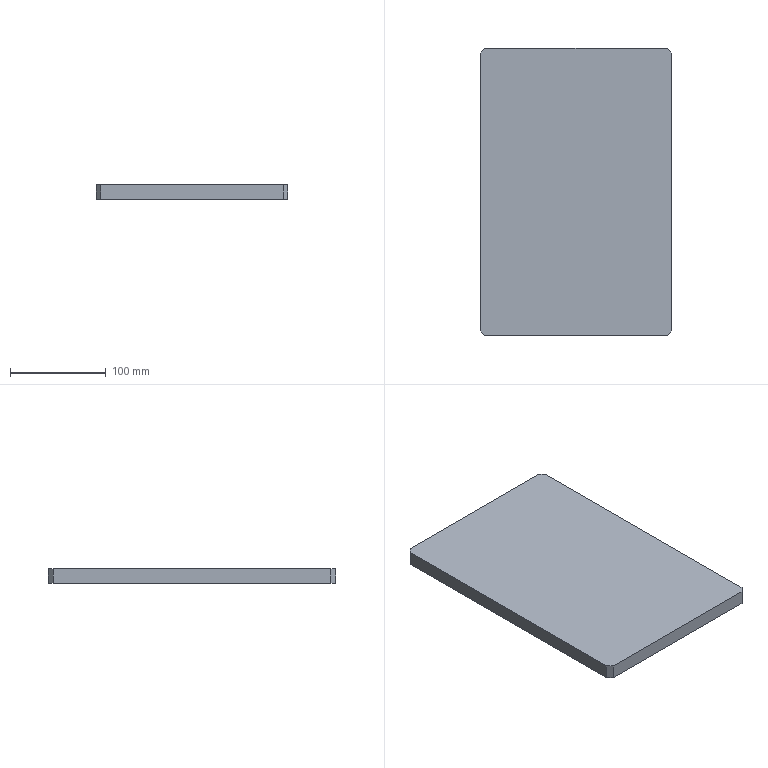Part | SolidWorks | features Chamfer 1, Extrusion 1 | 1 solid | 10 faces | box 200 x 300 x 15 mm | volume 899250 mm3 | plane 10
STEP:
#1=CARTESIAN_POINT('',(100.,-145.,7.5));
#2=VERTEX_POINT('',#1);
#3=CARTESIAN_POINT('',(100.,145.,7.5));
#4=VERTEX_POINT('',#3);
#5=CARTESIAN_POINT('',(100.,-150.,7.5));
#6=DIRECTION('',(0.,1.,0.));
#7=VECTOR('',#6,1000.);
#8=LINE('',#5,#7);
#9=EDGE_CURVE('',#2,#4,#8,.T.);
#10=ORIENTED_EDGE('',*,*,#9,.F.);
#11=CARTESIAN_POINT('',(100.,-145.,-7.5));
#12=VERTEX_POINT('',#11);
#13=CARTESIAN_POINT('',(100.,-145.,7.5));
#14=DIRECTION('',(0.,0.,-1.));
#15=VECTOR('',#14,1000.);
#16=LINE('',#13,#15);
#17=EDGE_CURVE('',#2,#12,#16,.T.);
#18=ORIENTED_EDGE('',*,*,#17,.T.);
#19=CARTESIAN_POINT('',(100.,145.,-7.5));
#20=VERTEX_POINT('',#19);
#21=CARTESIAN_POINT('',(100.,-150.,-7.5));
#22=DIRECTION('',(0.,1.,0.));
#23=VECTOR('',#22,1000.);
#24=LINE('',#21,#23);
#25=EDGE_CURVE('',#12,#20,#24,.T.);
#26=ORIENTED_EDGE('',*,*,#25,.T.);
#27=CARTESIAN_POINT('',(100.,145.,7.5));
#28=DIRECTION('',(0.,0.,1.));
#29=VECTOR('',#28,1000.);
#30=LINE('',#27,#29);
#31=EDGE_CURVE('',#20,#4,#30,.T.);
#32=ORIENTED_EDGE('',*,*,#31,.T.);
#33=EDGE_LOOP('',(#10,#18,#26,#32));
#34=FACE_OUTER_BOUND('',#33,.T.);
#35=CARTESIAN_POINT('',(100.,-150.,7.5));
#36=DIRECTION('',(-1.,0.,0.));
#37=DIRECTION('',(0.,0.,1.));
#38=AXIS2_PLACEMENT_3D('',#35,#36,#37);
#39=PLANE('',#38);
#40=ADVANCED_FACE('',(#34),#39,.F.);
#41=CARTESIAN_POINT('',(95.,150.,-7.5));
#42=VERTEX_POINT('',#41);
#43=CARTESIAN_POINT('',(-95.,150.,-7.5));
#44=VERTEX_POINT('',#43);
#45=CARTESIAN_POINT('',(-100.,150.,-7.5));
#46=DIRECTION('',(-1.,0.,0.));
#47=VECTOR('',#46,1000.);
#48=LINE('',#45,#47);
#49=EDGE_CURVE('',#42,#44,#48,.T.);
#50=ORIENTED_EDGE('',*,*,#49,.T.);
#51=CARTESIAN_POINT('',(-95.,150.,7.5));
#52=VERTEX_POINT('',#51);
#53=CARTESIAN_POINT('',(-95.,150.,7.5));
#54=DIRECTION('',(0.,0.,1.));
#55=VECTOR('',#54,1000.);
#56=LINE('',#53,#55);
#57=EDGE_CURVE('',#44,#52,#56,.T.);
#58=ORIENTED_EDGE('',*,*,#57,.T.);
#59=CARTESIAN_POINT('',(95.,150.,7.5));
#60=VERTEX_POINT('',#59);
#61=CARTESIAN_POINT('',(-100.,150.,7.5));
#62=DIRECTION('',(-1.,0.,0.));
#63=VECTOR('',#62,1000.);
#64=LINE('',#61,#63);
#65=EDGE_CURVE('',#60,#52,#64,.T.);
#66=ORIENTED_EDGE('',*,*,#65,.F.);
#67=CARTESIAN_POINT('',(95.,150.,7.5));
#68=DIRECTION('',(0.,0.,-1.));
#69=VECTOR('',#68,1000.);
#70=LINE('',#67,#69);
#71=EDGE_CURVE('',#60,#42,#70,.T.);
#72=ORIENTED_EDGE('',*,*,#71,.T.);
#73=EDGE_LOOP('',(#50,#58,#66,#72));
#74=FACE_OUTER_BOUND('',#73,.T.);
#75=CARTESIAN_POINT('',(-100.,150.,7.5));
#76=DIRECTION('',(0.,-1.,0.));
#77=DIRECTION('',(0.,0.,-1.));
#78=AXIS2_PLACEMENT_3D('',#75,#76,#77);
#79=PLANE('',#78);
#80=ADVANCED_FACE('',(#74),#79,.F.);
#81=CARTESIAN_POINT('',(-100.,145.,-7.5));
#82=VERTEX_POINT('',#81);
#83=CARTESIAN_POINT('',(-100.,-145.,-7.5));
#84=VERTEX_POINT('',#83);
#85=CARTESIAN_POINT('',(-100.,-150.,-7.5));
#86=DIRECTION('',(0.,-1.,0.));
#87=VECTOR('',#86,1000.);
#88=LINE('',#85,#87);
#89=EDGE_CURVE('',#82,#84,#88,.T.);
#90=ORIENTED_EDGE('',*,*,#89,.T.);
#91=CARTESIAN_POINT('',(-100.,-145.,7.5));
#92=VERTEX_POINT('',#91);
#93=CARTESIAN_POINT('',(-100.,-145.,7.5));
#94=DIRECTION('',(0.,0.,1.));
#95=VECTOR('',#94,1000.);
#96=LINE('',#93,#95);
#97=EDGE_CURVE('',#84,#92,#96,.T.);
#98=ORIENTED_EDGE('',*,*,#97,.T.);
#99=CARTESIAN_POINT('',(-100.,145.,7.5));
#100=VERTEX_POINT('',#99);
#101=CARTESIAN_POINT('',(-100.,-150.,7.5));
#102=DIRECTION('',(0.,-1.,0.));
#103=VECTOR('',#102,1000.);
#104=LINE('',#101,#103);
#105=EDGE_CURVE('',#100,#92,#104,.T.);
#106=ORIENTED_EDGE('',*,*,#105,.F.);
#107=CARTESIAN_POINT('',(-100.,145.,7.5));
#108=DIRECTION('',(0.,0.,-1.));
#109=VECTOR('',#108,1000.);
#110=LINE('',#107,#109);
#111=EDGE_CURVE('',#100,#82,#110,.T.);
#112=ORIENTED_EDGE('',*,*,#111,.T.);
#113=EDGE_LOOP('',(#90,#98,#106,#112));
#114=FACE_OUTER_BOUND('',#113,.T.);
#115=CARTESIAN_POINT('',(-100.,-150.,7.5));
#116=DIRECTION('',(1.,0.,0.));
#117=DIRECTION('',(0.,0.,-1.));
#118=AXIS2_PLACEMENT_3D('',#115,#116,#117);
#119=PLANE('',#118);
#120=ADVANCED_FACE('',(#114),#119,.F.);
#121=CARTESIAN_POINT('',(-95.,-150.,7.5));
#122=VERTEX_POINT('',#121);
#123=CARTESIAN_POINT('',(95.,-150.,7.5));
#124=VERTEX_POINT('',#123);
#125=CARTESIAN_POINT('',(-100.,-150.,7.5));
#126=DIRECTION('',(1.,0.,0.));
#127=VECTOR('',#126,1000.);
#128=LINE('',#125,#127);
#129=EDGE_CURVE('',#122,#124,#128,.T.);
#130=ORIENTED_EDGE('',*,*,#129,.F.);
#131=CARTESIAN_POINT('',(-95.,-150.,-7.5));
#132=VERTEX_POINT('',#131);
#133=CARTESIAN_POINT('',(-95.,-150.,7.5));
#134=DIRECTION('',(0.,0.,-1.));
#135=VECTOR('',#134,1000.);
#136=LINE('',#133,#135);
#137=EDGE_CURVE('',#122,#132,#136,.T.);
#138=ORIENTED_EDGE('',*,*,#137,.T.);
#139=CARTESIAN_POINT('',(95.,-150.,-7.5));
#140=VERTEX_POINT('',#139);
#141=CARTESIAN_POINT('',(-100.,-150.,-7.5));
#142=DIRECTION('',(1.,0.,0.));
#143=VECTOR('',#142,1000.);
#144=LINE('',#141,#143);
#145=EDGE_CURVE('',#132,#140,#144,.T.);
#146=ORIENTED_EDGE('',*,*,#145,.T.);
#147=CARTESIAN_POINT('',(95.,-150.,7.5));
#148=DIRECTION('',(0.,0.,1.));
#149=VECTOR('',#148,1000.);
#150=LINE('',#147,#149);
#151=EDGE_CURVE('',#140,#124,#150,.T.);
#152=ORIENTED_EDGE('',*,*,#151,.T.);
#153=EDGE_LOOP('',(#130,#138,#146,#152));
#154=FACE_OUTER_BOUND('',#153,.T.);
#155=CARTESIAN_POINT('',(-100.,-150.,7.5));
#156=DIRECTION('',(0.,1.,0.));
#157=DIRECTION('',(0.,0.,1.));
#158=AXIS2_PLACEMENT_3D('',#155,#156,#157);
#159=PLANE('',#158);
#160=ADVANCED_FACE('',(#154),#159,.F.);
#161=ORIENTED_EDGE('',*,*,#105,.T.);
#162=CARTESIAN_POINT('',(-95.,-150.,7.5));
#163=DIRECTION('',(0.7071,-0.7071,0.));
#164=VECTOR('',#163,1000.);
#165=LINE('',#162,#164);
#166=EDGE_CURVE('',#92,#122,#165,.T.);
#167=ORIENTED_EDGE('',*,*,#166,.T.);
#168=ORIENTED_EDGE('',*,*,#129,.T.);
#169=CARTESIAN_POINT('',(100.,-145.,7.5));
#170=DIRECTION('',(0.7071,0.7071,0.));
#171=VECTOR('',#170,1000.);
#172=LINE('',#169,#171);
#173=EDGE_CURVE('',#124,#2,#172,.T.);
#174=ORIENTED_EDGE('',*,*,#173,.T.);
#175=ORIENTED_EDGE('',*,*,#9,.T.);
#176=CARTESIAN_POINT('',(95.,150.,7.5));
#177=DIRECTION('',(-0.7071,0.7071,0.));
#178=VECTOR('',#177,1000.);
#179=LINE('',#176,#178);
#180=EDGE_CURVE('',#4,#60,#179,.T.);
#181=ORIENTED_EDGE('',*,*,#180,.T.);
#182=ORIENTED_EDGE('',*,*,#65,.T.);
#183=CARTESIAN_POINT('',(-100.,145.,7.5));
#184=DIRECTION('',(-0.7071,-0.7071,0.));
#185=VECTOR('',#184,1000.);
#186=LINE('',#183,#185);
#187=EDGE_CURVE('',#52,#100,#186,.T.);
#188=ORIENTED_EDGE('',*,*,#187,.T.);
#189=EDGE_LOOP('',(#161,#167,#168,#174,#175,#181,#182,#188));
#190=FACE_OUTER_BOUND('',#189,.T.);
#191=CARTESIAN_POINT('',(0.,0.,7.5));
#192=DIRECTION('',(0.,0.,-1.));
#193=DIRECTION('',(-1.,0.,0.));
#194=AXIS2_PLACEMENT_3D('',#191,#192,#193);
#195=PLANE('',#194);
#196=ADVANCED_FACE('',(#190),#195,.F.);
#197=ORIENTED_EDGE('',*,*,#145,.F.);
#198=CARTESIAN_POINT('',(-122.5,-122.5,-7.5));
#199=DIRECTION('',(-0.7071,0.7071,0.));
#200=VECTOR('',#199,1000.);
#201=LINE('',#198,#200);
#202=EDGE_CURVE('',#132,#84,#201,.T.);
#203=ORIENTED_EDGE('',*,*,#202,.T.);
#204=ORIENTED_EDGE('',*,*,#89,.F.);
#205=CARTESIAN_POINT('',(-122.5,122.5,-7.5));
#206=DIRECTION('',(0.7071,0.7071,0.));
#207=VECTOR('',#206,1000.);
#208=LINE('',#205,#207);
#209=EDGE_CURVE('',#82,#44,#208,.T.);
#210=ORIENTED_EDGE('',*,*,#209,.T.);
#211=ORIENTED_EDGE('',*,*,#49,.F.);
#212=CARTESIAN_POINT('',(122.5,122.5,-7.5));
#213=DIRECTION('',(0.7071,-0.7071,0.));
#214=VECTOR('',#213,1000.);
#215=LINE('',#212,#214);
#216=EDGE_CURVE('',#42,#20,#215,.T.);
#217=ORIENTED_EDGE('',*,*,#216,.T.);
#218=ORIENTED_EDGE('',*,*,#25,.F.);
#219=CARTESIAN_POINT('',(122.5,-122.5,-7.5));
#220=DIRECTION('',(-0.7071,-0.7071,0.));
#221=VECTOR('',#220,1000.);
#222=LINE('',#219,#221);
#223=EDGE_CURVE('',#12,#140,#222,.T.);
#224=ORIENTED_EDGE('',*,*,#223,.T.);
#225=EDGE_LOOP('',(#197,#203,#204,#210,#211,#217,#218,#224));
#226=FACE_OUTER_BOUND('',#225,.T.);
#227=CARTESIAN_POINT('',(0.,0.,-7.5));
#228=DIRECTION('',(0.,0.,-1.));
#229=DIRECTION('',(-1.,0.,0.));
#230=AXIS2_PLACEMENT_3D('',#227,#228,#229);
#231=PLANE('',#230);
#232=ADVANCED_FACE('',(#226),#231,.T.);
#233=ORIENTED_EDGE('',*,*,#166,.F.);
#234=ORIENTED_EDGE('',*,*,#97,.F.);
#235=ORIENTED_EDGE('',*,*,#202,.F.);
#236=ORIENTED_EDGE('',*,*,#137,.F.);
#237=EDGE_LOOP('',(#233,#234,#235,#236));
#238=FACE_OUTER_BOUND('',#237,.T.);
#239=CARTESIAN_POINT('',(-95.,-150.,7.5));
#240=DIRECTION('',(0.7071,0.7071,0.));
#241=DIRECTION('',(0.,0.,-1.));
#242=AXIS2_PLACEMENT_3D('',#239,#240,#241);
#243=PLANE('',#242);
#244=ADVANCED_FACE('',(#238),#243,.F.);
#245=ORIENTED_EDGE('',*,*,#187,.F.);
#246=ORIENTED_EDGE('',*,*,#57,.F.);
#247=ORIENTED_EDGE('',*,*,#209,.F.);
#248=ORIENTED_EDGE('',*,*,#111,.F.);
#249=EDGE_LOOP('',(#245,#246,#247,#248));
#250=FACE_OUTER_BOUND('',#249,.T.);
#251=CARTESIAN_POINT('',(-100.,145.,7.5));
#252=DIRECTION('',(0.7071,-0.7071,0.));
#253=DIRECTION('',(0.,0.,-1.));
#254=AXIS2_PLACEMENT_3D('',#251,#252,#253);
#255=PLANE('',#254);
#256=ADVANCED_FACE('',(#250),#255,.F.);
#257=ORIENTED_EDGE('',*,*,#173,.F.);
#258=ORIENTED_EDGE('',*,*,#151,.F.);
#259=ORIENTED_EDGE('',*,*,#223,.F.);
#260=ORIENTED_EDGE('',*,*,#17,.F.);
#261=EDGE_LOOP('',(#257,#258,#259,#260));
#262=FACE_OUTER_BOUND('',#261,.T.);
#263=CARTESIAN_POINT('',(100.,-145.,7.5));
#264=DIRECTION('',(-0.7071,0.7071,0.));
#265=DIRECTION('',(0.,0.,-1.));
#266=AXIS2_PLACEMENT_3D('',#263,#264,#265);
#267=PLANE('',#266);
#268=ADVANCED_FACE('',(#262),#267,.F.);
#269=ORIENTED_EDGE('',*,*,#180,.F.);
#270=ORIENTED_EDGE('',*,*,#31,.F.);
#271=ORIENTED_EDGE('',*,*,#216,.F.);
#272=ORIENTED_EDGE('',*,*,#71,.F.);
#273=EDGE_LOOP('',(#269,#270,#271,#272));
#274=FACE_OUTER_BOUND('',#273,.T.);
#275=CARTESIAN_POINT('',(95.,150.,7.5));
#276=DIRECTION('',(-0.7071,-0.7071,0.));
#277=DIRECTION('',(0.,0.,-1.));
#278=AXIS2_PLACEMENT_3D('',#275,#276,#277);
#279=PLANE('',#278);
#280=ADVANCED_FACE('',(#274),#279,.F.);
#281=CLOSED_SHELL('',(#40,#80,#120,#160,#196,#232,#244,#256,#268,#280));
#282=MANIFOLD_SOLID_BREP('',#281);
#283=CARTESIAN_POINT('',(0.,0.,0.));
#284=DIRECTION('',(0.,0.,1.));
#285=DIRECTION('',(1.,0.,0.));
#286=AXIS2_PLACEMENT_3D('',#283,#284,#285);
#287=(LENGTH_UNIT()NAMED_UNIT(*)SI_UNIT(.MILLI.,.METRE.));
#288=UNCERTAINTY_MEASURE_WITH_UNIT(LENGTH_MEASURE(0.00001),#287,'','');
#289=(NAMED_UNIT(*)PLANE_ANGLE_UNIT()SI_UNIT($,.RADIAN.));
#290=(NAMED_UNIT(*)SI_UNIT($,.STERADIAN.)SOLID_ANGLE_UNIT());
#291=(GEOMETRIC_REPRESENTATION_CONTEXT(3)GLOBAL_UNCERTAINTY_ASSIGNED_CONTEXT((#288))GLOBAL_UNIT_ASSIGNED_CONTEXT((#287,#289,#290))REPRESENTATION_CONTEXT('',''));
#292=ADVANCED_BREP_SHAPE_REPRESENTATION('',(#282,#286),#291);